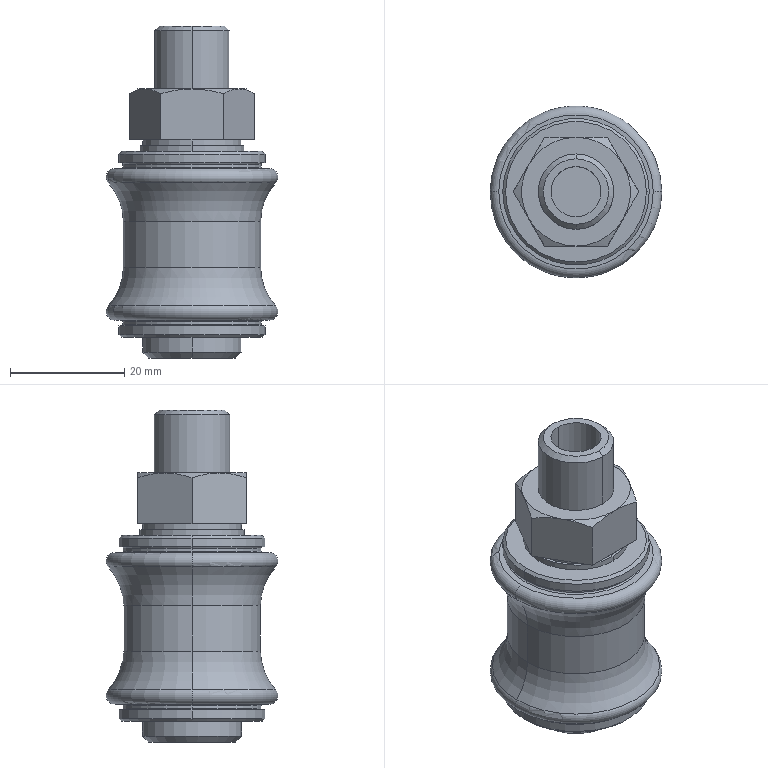Part | SolidWorks | features BaseBody 2 | 2 solids | 78 faces | box 30 x 30 x 58 mm | volume 20249 mm3 | cylinder 24 | plane 20 | torus 18 | cone 16 | commonest cylinder face diameters 17.3 x4 18.3 x4 24.2 x4 25.6 x4 8.771 x2 11.445 x2